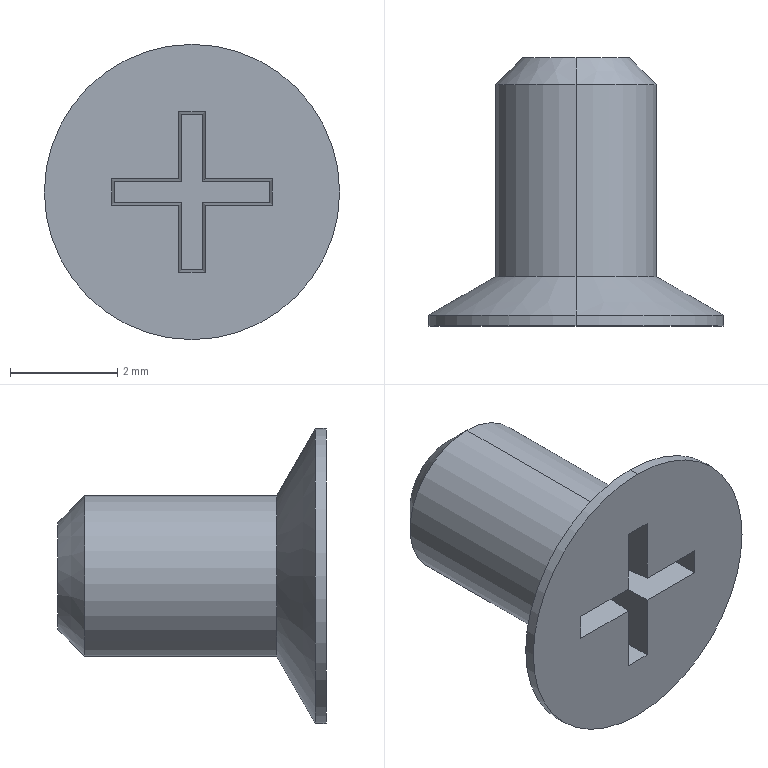Part | SolidWorks | features BaseBody 1 | 1 solid | 23 faces | box 5.5 x 5 x 5.5 mm | volume 40.626 mm3 | plane 15 | cylinder 4 | cone 4 | commonest cylinder face diameters 3 x2 5.5 x2
STEP:
#1=CARTESIAN_POINT('',(0.,0.2,-2.75));
#2=VERTEX_POINT('',#1);
#3=CARTESIAN_POINT('',(0.,0.2,2.75));
#4=VERTEX_POINT('',#3);
#5=CARTESIAN_POINT('',(0.,0.2,0.));
#6=DIRECTION('',(0.,-1.,0.));
#7=DIRECTION('',(0.,0.,-1.));
#8=AXIS2_PLACEMENT_3D('',#5,#6,#7);
#9=CIRCLE('',#8,2.75);
#10=EDGE_CURVE('',#2,#4,#9,.T.);
#11=ORIENTED_EDGE('',*,*,#10,.T.);
#12=CARTESIAN_POINT('',(0.,0.,2.75));
#13=VERTEX_POINT('',#12);
#14=CARTESIAN_POINT('',(0.,0.,2.75));
#15=DIRECTION('',(0.,-1.,0.));
#16=VECTOR('',#15,1000.);
#17=LINE('',#14,#16);
#18=EDGE_CURVE('',#4,#13,#17,.T.);
#19=ORIENTED_EDGE('',*,*,#18,.T.);
#20=CARTESIAN_POINT('',(0.,0.,-2.75));
#21=VERTEX_POINT('',#20);
#22=CARTESIAN_POINT('',(0.,0.,0.));
#23=DIRECTION('',(0.,-1.,0.));
#24=DIRECTION('',(0.,0.,-1.));
#25=AXIS2_PLACEMENT_3D('',#22,#23,#24);
#26=CIRCLE('',#25,2.75);
#27=EDGE_CURVE('',#21,#13,#26,.T.);
#28=ORIENTED_EDGE('',*,*,#27,.F.);
#29=CARTESIAN_POINT('',(0.,0.,-2.75));
#30=DIRECTION('',(0.,-1.,0.));
#31=VECTOR('',#30,1000.);
#32=LINE('',#29,#31);
#33=EDGE_CURVE('',#2,#21,#32,.T.);
#34=ORIENTED_EDGE('',*,*,#33,.F.);
#35=EDGE_LOOP('',(#11,#19,#28,#34));
#36=FACE_OUTER_BOUND('',#35,.T.);
#37=CARTESIAN_POINT('',(0.,0.,0.));
#38=DIRECTION('',(0.,-1.,0.));
#39=DIRECTION('',(0.,0.,-1.));
#40=AXIS2_PLACEMENT_3D('',#37,#38,#39);
#41=CYLINDRICAL_SURFACE('',#40,2.75);
#42=ADVANCED_FACE('',(#36),#41,.T.);
#43=CARTESIAN_POINT('',(0.,0.9217,-1.5));
#44=VERTEX_POINT('',#43);
#45=CARTESIAN_POINT('',(0.,0.9217,1.5));
#46=VERTEX_POINT('',#45);
#47=CARTESIAN_POINT('',(0.,0.9217,0.));
#48=DIRECTION('',(0.,-1.,0.));
#49=DIRECTION('',(0.,0.,-1.));
#50=AXIS2_PLACEMENT_3D('',#47,#48,#49);
#51=CIRCLE('',#50,1.5);
#52=EDGE_CURVE('',#44,#46,#51,.T.);
#53=ORIENTED_EDGE('',*,*,#52,.T.);
#54=CARTESIAN_POINT('',(0.,0.2,2.75));
#55=DIRECTION('',(0.,-0.5,0.866));
#56=VECTOR('',#55,1000.);
#57=LINE('',#54,#56);
#58=EDGE_CURVE('',#46,#4,#57,.T.);
#59=ORIENTED_EDGE('',*,*,#58,.T.);
#60=ORIENTED_EDGE('',*,*,#10,.F.);
#61=CARTESIAN_POINT('',(0.,0.2,-2.75));
#62=DIRECTION('',(0.,-0.5,-0.866));
#63=VECTOR('',#62,1000.);
#64=LINE('',#61,#63);
#65=EDGE_CURVE('',#44,#2,#64,.T.);
#66=ORIENTED_EDGE('',*,*,#65,.F.);
#67=EDGE_LOOP('',(#53,#59,#60,#66));
#68=FACE_OUTER_BOUND('',#67,.T.);
#69=CARTESIAN_POINT('',(0.,0.2,0.));
#70=DIRECTION('',(0.,-1.,0.));
#71=DIRECTION('',(0.,0.,-1.));
#72=AXIS2_PLACEMENT_3D('',#69,#70,#71);
#73=CONICAL_SURFACE('',#72,2.75,1.047);
#74=ADVANCED_FACE('',(#68),#73,.T.);
#75=CARTESIAN_POINT('',(0.,4.5,-1.5));
#76=VERTEX_POINT('',#75);
#77=CARTESIAN_POINT('',(0.,4.5,1.5));
#78=VERTEX_POINT('',#77);
#79=CARTESIAN_POINT('',(0.,4.5,0.));
#80=DIRECTION('',(0.,-1.,0.));
#81=DIRECTION('',(0.,0.,-1.));
#82=AXIS2_PLACEMENT_3D('',#79,#80,#81);
#83=CIRCLE('',#82,1.5);
#84=EDGE_CURVE('',#76,#78,#83,.T.);
#85=ORIENTED_EDGE('',*,*,#84,.T.);
#86=CARTESIAN_POINT('',(0.,0.,1.5));
#87=DIRECTION('',(0.,-1.,0.));
#88=VECTOR('',#87,1000.);
#89=LINE('',#86,#88);
#90=EDGE_CURVE('',#78,#46,#89,.T.);
#91=ORIENTED_EDGE('',*,*,#90,.T.);
#92=ORIENTED_EDGE('',*,*,#52,.F.);
#93=CARTESIAN_POINT('',(0.,0.,-1.5));
#94=DIRECTION('',(0.,-1.,0.));
#95=VECTOR('',#94,1000.);
#96=LINE('',#93,#95);
#97=EDGE_CURVE('',#76,#44,#96,.T.);
#98=ORIENTED_EDGE('',*,*,#97,.F.);
#99=EDGE_LOOP('',(#85,#91,#92,#98));
#100=FACE_OUTER_BOUND('',#99,.T.);
#101=CARTESIAN_POINT('',(0.,0.,0.));
#102=DIRECTION('',(0.,-1.,0.));
#103=DIRECTION('',(0.,0.,-1.));
#104=AXIS2_PLACEMENT_3D('',#101,#102,#103);
#105=CYLINDRICAL_SURFACE('',#104,1.5);
#106=ADVANCED_FACE('',(#100),#105,.T.);
#107=CARTESIAN_POINT('',(0.,5.,-1.));
#108=VERTEX_POINT('',#107);
#109=CARTESIAN_POINT('',(0.,5.,1.));
#110=VERTEX_POINT('',#109);
#111=CARTESIAN_POINT('',(0.,5.,0.));
#112=DIRECTION('',(0.,-1.,0.));
#113=DIRECTION('',(0.,0.,-1.));
#114=AXIS2_PLACEMENT_3D('',#111,#112,#113);
#115=CIRCLE('',#114,1.);
#116=EDGE_CURVE('',#108,#110,#115,.T.);
#117=ORIENTED_EDGE('',*,*,#116,.T.);
#118=CARTESIAN_POINT('',(0.,4.5,1.5));
#119=DIRECTION('',(0.,-0.7071,0.7071));
#120=VECTOR('',#119,1000.);
#121=LINE('',#118,#120);
#122=EDGE_CURVE('',#110,#78,#121,.T.);
#123=ORIENTED_EDGE('',*,*,#122,.T.);
#124=ORIENTED_EDGE('',*,*,#84,.F.);
#125=CARTESIAN_POINT('',(0.,4.5,-1.5));
#126=DIRECTION('',(0.,-0.7071,-0.7071));
#127=VECTOR('',#126,1000.);
#128=LINE('',#125,#127);
#129=EDGE_CURVE('',#108,#76,#128,.T.);
#130=ORIENTED_EDGE('',*,*,#129,.F.);
#131=EDGE_LOOP('',(#117,#123,#124,#130));
#132=FACE_OUTER_BOUND('',#131,.T.);
#133=CARTESIAN_POINT('',(0.,4.5,0.));
#134=DIRECTION('',(0.,-1.,0.));
#135=DIRECTION('',(0.,0.,-1.));
#136=AXIS2_PLACEMENT_3D('',#133,#134,#135);
#137=CONICAL_SURFACE('',#136,1.5,0.7854);
#138=ADVANCED_FACE('',(#132),#137,.T.);
#139=ORIENTED_EDGE('',*,*,#27,.T.);
#140=CARTESIAN_POINT('',(0.,0.,0.));
#141=DIRECTION('',(0.,-1.,0.));
#142=DIRECTION('',(0.,0.,-1.));
#143=AXIS2_PLACEMENT_3D('',#140,#141,#142);
#144=CIRCLE('',#143,2.75);
#145=EDGE_CURVE('',#13,#21,#144,.T.);
#146=ORIENTED_EDGE('',*,*,#145,.T.);
#147=EDGE_LOOP('',(#139,#146));
#148=FACE_OUTER_BOUND('',#147,.T.);
#149=CARTESIAN_POINT('',(-1.5,0.,0.25));
#150=VERTEX_POINT('',#149);
#151=CARTESIAN_POINT('',(-0.25,0.,0.25));
#152=VERTEX_POINT('',#151);
#153=CARTESIAN_POINT('',(2.75,0.,0.25));
#154=DIRECTION('',(1.,0.,0.));
#155=VECTOR('',#154,1000.);
#156=LINE('',#153,#155);
#157=EDGE_CURVE('',#150,#152,#156,.T.);
#158=ORIENTED_EDGE('',*,*,#157,.T.);
#159=CARTESIAN_POINT('',(-0.25,0.,1.5));
#160=VERTEX_POINT('',#159);
#161=CARTESIAN_POINT('',(-0.25,0.,0.));
#162=DIRECTION('',(0.,0.,1.));
#163=VECTOR('',#162,1000.);
#164=LINE('',#161,#163);
#165=EDGE_CURVE('',#152,#160,#164,.T.);
#166=ORIENTED_EDGE('',*,*,#165,.T.);
#167=CARTESIAN_POINT('',(0.25,0.,1.5));
#168=VERTEX_POINT('',#167);
#169=CARTESIAN_POINT('',(2.75,0.,1.5));
#170=DIRECTION('',(1.,0.,0.));
#171=VECTOR('',#170,1000.);
#172=LINE('',#169,#171);
#173=EDGE_CURVE('',#160,#168,#172,.T.);
#174=ORIENTED_EDGE('',*,*,#173,.T.);
#175=CARTESIAN_POINT('',(0.25,0.,0.25));
#176=VERTEX_POINT('',#175);
#177=CARTESIAN_POINT('',(0.25,0.,0.));
#178=DIRECTION('',(0.,0.,-1.));
#179=VECTOR('',#178,1000.);
#180=LINE('',#177,#179);
#181=EDGE_CURVE('',#168,#176,#180,.T.);
#182=ORIENTED_EDGE('',*,*,#181,.T.);
#183=CARTESIAN_POINT('',(1.5,0.,0.25));
#184=VERTEX_POINT('',#183);
#185=CARTESIAN_POINT('',(2.75,0.,0.25));
#186=DIRECTION('',(1.,0.,0.));
#187=VECTOR('',#186,1000.);
#188=LINE('',#185,#187);
#189=EDGE_CURVE('',#176,#184,#188,.T.);
#190=ORIENTED_EDGE('',*,*,#189,.T.);
#191=CARTESIAN_POINT('',(1.5,0.,-0.25));
#192=VERTEX_POINT('',#191);
#193=CARTESIAN_POINT('',(1.5,0.,0.));
#194=DIRECTION('',(0.,0.,-1.));
#195=VECTOR('',#194,1000.);
#196=LINE('',#193,#195);
#197=EDGE_CURVE('',#184,#192,#196,.T.);
#198=ORIENTED_EDGE('',*,*,#197,.T.);
#199=CARTESIAN_POINT('',(0.25,0.,-0.25));
#200=VERTEX_POINT('',#199);
#201=CARTESIAN_POINT('',(2.75,0.,-0.25));
#202=DIRECTION('',(-1.,0.,0.));
#203=VECTOR('',#202,1000.);
#204=LINE('',#201,#203);
#205=EDGE_CURVE('',#192,#200,#204,.T.);
#206=ORIENTED_EDGE('',*,*,#205,.T.);
#207=CARTESIAN_POINT('',(0.25,0.,-1.5));
#208=VERTEX_POINT('',#207);
#209=CARTESIAN_POINT('',(0.25,0.,0.));
#210=DIRECTION('',(0.,0.,-1.));
#211=VECTOR('',#210,1000.);
#212=LINE('',#209,#211);
#213=EDGE_CURVE('',#200,#208,#212,.T.);
#214=ORIENTED_EDGE('',*,*,#213,.T.);
#215=CARTESIAN_POINT('',(-0.25,0.,-1.5));
#216=VERTEX_POINT('',#215);
#217=CARTESIAN_POINT('',(2.75,0.,-1.5));
#218=DIRECTION('',(-1.,0.,0.));
#219=VECTOR('',#218,1000.);
#220=LINE('',#217,#219);
#221=EDGE_CURVE('',#208,#216,#220,.T.);
#222=ORIENTED_EDGE('',*,*,#221,.T.);
#223=CARTESIAN_POINT('',(-0.25,0.,-0.25));
#224=VERTEX_POINT('',#223);
#225=CARTESIAN_POINT('',(-0.25,0.,0.));
#226=DIRECTION('',(0.,0.,1.));
#227=VECTOR('',#226,1000.);
#228=LINE('',#225,#227);
#229=EDGE_CURVE('',#216,#224,#228,.T.);
#230=ORIENTED_EDGE('',*,*,#229,.T.);
#231=CARTESIAN_POINT('',(-1.5,0.,-0.25));
#232=VERTEX_POINT('',#231);
#233=CARTESIAN_POINT('',(2.75,0.,-0.25));
#234=DIRECTION('',(-1.,0.,0.));
#235=VECTOR('',#234,1000.);
#236=LINE('',#233,#235);
#237=EDGE_CURVE('',#224,#232,#236,.T.);
#238=ORIENTED_EDGE('',*,*,#237,.T.);
#239=CARTESIAN_POINT('',(-1.5,0.,0.));
#240=DIRECTION('',(0.,0.,1.));
#241=VECTOR('',#240,1000.);
#242=LINE('',#239,#241);
#243=EDGE_CURVE('',#232,#150,#242,.T.);
#244=ORIENTED_EDGE('',*,*,#243,.T.);
#245=EDGE_LOOP('',(#158,#166,#174,#182,#190,#198,#206,#214,#222,#230,#238,#244));
#246=FACE_BOUND('',#245,.T.);
#247=CARTESIAN_POINT('',(2.75,0.,0.));
#248=DIRECTION('',(0.,-1.,0.));
#249=DIRECTION('',(0.,0.,-1.));
#250=AXIS2_PLACEMENT_3D('',#247,#248,#249);
#251=PLANE('',#250);
#252=ADVANCED_FACE('',(#148,#246),#251,.T.);
#253=ORIENTED_EDGE('',*,*,#18,.F.);
#254=CARTESIAN_POINT('',(0.,0.2,0.));
#255=DIRECTION('',(0.,-1.,0.));
#256=DIRECTION('',(0.,0.,-1.));
#257=AXIS2_PLACEMENT_3D('',#254,#255,#256);
#258=CIRCLE('',#257,2.75);
#259=EDGE_CURVE('',#4,#2,#258,.T.);
#260=ORIENTED_EDGE('',*,*,#259,.T.);
#261=ORIENTED_EDGE('',*,*,#33,.T.);
#262=ORIENTED_EDGE('',*,*,#145,.F.);
#263=EDGE_LOOP('',(#253,#260,#261,#262));
#264=FACE_OUTER_BOUND('',#263,.T.);
#265=CARTESIAN_POINT('',(0.,0.,0.));
#266=DIRECTION('',(0.,-1.,0.));
#267=DIRECTION('',(0.,0.,-1.));
#268=AXIS2_PLACEMENT_3D('',#265,#266,#267);
#269=CYLINDRICAL_SURFACE('',#268,2.75);
#270=ADVANCED_FACE('',(#264),#269,.T.);
#271=CARTESIAN_POINT('',(-0.1976,1.,0.1976));
#272=VERTEX_POINT('',#271);
#273=CARTESIAN_POINT('',(-0.1976,1.,0.1976));
#274=DIRECTION('',(-0.05226,-0.9973,0.05226));
#275=VECTOR('',#274,1000.);
#276=LINE('',#273,#275);
#277=EDGE_CURVE('',#272,#152,#276,.T.);
#278=ORIENTED_EDGE('',*,*,#277,.F.);
#279=CARTESIAN_POINT('',(-0.1976,1.,1.448));
#280=VERTEX_POINT('',#279);
#281=CARTESIAN_POINT('',(-0.1976,1.,0.25));
#282=DIRECTION('',(0.,0.,-1.));
#283=VECTOR('',#282,1000.);
#284=LINE('',#281,#283);
#285=EDGE_CURVE('',#280,#272,#284,.T.);
#286=ORIENTED_EDGE('',*,*,#285,.F.);
#287=CARTESIAN_POINT('',(-0.25,0.,1.5));
#288=DIRECTION('',(0.05226,0.9973,-0.05226));
#289=VECTOR('',#288,1000.);
#290=LINE('',#287,#289);
#291=EDGE_CURVE('',#160,#280,#290,.T.);
#292=ORIENTED_EDGE('',*,*,#291,.F.);
#293=ORIENTED_EDGE('',*,*,#165,.F.);
#294=EDGE_LOOP('',(#278,#286,#292,#293));
#295=FACE_OUTER_BOUND('',#294,.T.);
#296=CARTESIAN_POINT('',(-0.25,0.,0.25));
#297=DIRECTION('',(-0.9986,0.05234,0.));
#298=DIRECTION('',(-0.05234,-0.9986,0.));
#299=AXIS2_PLACEMENT_3D('',#296,#297,#298);
#300=PLANE('',#299);
#301=ADVANCED_FACE('',(#295),#300,.F.);
#302=CARTESIAN_POINT('',(-1.448,1.,0.1976));
#303=VERTEX_POINT('',#302);
#304=CARTESIAN_POINT('',(-1.448,1.,0.1976));
#305=DIRECTION('',(-0.05226,-0.9973,0.05226));
#306=VECTOR('',#305,1000.);
#307=LINE('',#304,#306);
#308=EDGE_CURVE('',#303,#150,#307,.T.);
#309=ORIENTED_EDGE('',*,*,#308,.F.);
#310=CARTESIAN_POINT('',(-1.5,1.,0.1976));
#311=DIRECTION('',(-1.,0.,0.));
#312=VECTOR('',#311,1000.);
#313=LINE('',#310,#312);
#314=EDGE_CURVE('',#272,#303,#313,.T.);
#315=ORIENTED_EDGE('',*,*,#314,.F.);
#316=ORIENTED_EDGE('',*,*,#277,.T.);
#317=ORIENTED_EDGE('',*,*,#157,.F.);
#318=EDGE_LOOP('',(#309,#315,#316,#317));
#319=FACE_OUTER_BOUND('',#318,.T.);
#320=CARTESIAN_POINT('',(-1.5,0.,0.25));
#321=DIRECTION('',(0.,0.05234,0.9986));
#322=DIRECTION('',(0.,-0.9986,0.05234));
#323=AXIS2_PLACEMENT_3D('',#320,#321,#322);
#324=PLANE('',#323);
#325=ADVANCED_FACE('',(#319),#324,.F.);
#326=CARTESIAN_POINT('',(-1.448,1.,-0.1976));
#327=VERTEX_POINT('',#326);
#328=CARTESIAN_POINT('',(-1.448,1.,-0.1976));
#329=DIRECTION('',(-0.05226,-0.9973,-0.05226));
#330=VECTOR('',#329,1000.);
#331=LINE('',#328,#330);
#332=EDGE_CURVE('',#327,#232,#331,.T.);
#333=ORIENTED_EDGE('',*,*,#332,.F.);
#334=CARTESIAN_POINT('',(-1.448,1.,0.25));
#335=DIRECTION('',(0.,0.,-1.));
#336=VECTOR('',#335,1000.);
#337=LINE('',#334,#336);
#338=EDGE_CURVE('',#303,#327,#337,.T.);
#339=ORIENTED_EDGE('',*,*,#338,.F.);
#340=ORIENTED_EDGE('',*,*,#308,.T.);
#341=ORIENTED_EDGE('',*,*,#243,.F.);
#342=EDGE_LOOP('',(#333,#339,#340,#341));
#343=FACE_OUTER_BOUND('',#342,.T.);
#344=CARTESIAN_POINT('',(-1.5,0.,0.25));
#345=DIRECTION('',(-0.9986,0.05234,0.));
#346=DIRECTION('',(-0.05234,-0.9986,0.));
#347=AXIS2_PLACEMENT_3D('',#344,#345,#346);
#348=PLANE('',#347);
#349=ADVANCED_FACE('',(#343),#348,.F.);
#350=CARTESIAN_POINT('',(-0.1976,1.,-0.1976));
#351=VERTEX_POINT('',#350);
#352=CARTESIAN_POINT('',(-0.1976,1.,-0.1976));
#353=DIRECTION('',(-0.05226,-0.9973,-0.05226));
#354=VECTOR('',#353,1000.);
#355=LINE('',#352,#354);
#356=EDGE_CURVE('',#351,#224,#355,.T.);
#357=ORIENTED_EDGE('',*,*,#356,.F.);
#358=CARTESIAN_POINT('',(-1.5,1.,-0.1976));
#359=DIRECTION('',(1.,0.,0.));
#360=VECTOR('',#359,1000.);
#361=LINE('',#358,#360);
#362=EDGE_CURVE('',#327,#351,#361,.T.);
#363=ORIENTED_EDGE('',*,*,#362,.F.);
#364=ORIENTED_EDGE('',*,*,#332,.T.);
#365=ORIENTED_EDGE('',*,*,#237,.F.);
#366=EDGE_LOOP('',(#357,#363,#364,#365));
#367=FACE_OUTER_BOUND('',#366,.T.);
#368=CARTESIAN_POINT('',(-1.5,0.,-0.25));
#369=DIRECTION('',(0.,0.05234,-0.9986));
#370=DIRECTION('',(0.,0.9986,0.05234));
#371=AXIS2_PLACEMENT_3D('',#368,#369,#370);
#372=PLANE('',#371);
#373=ADVANCED_FACE('',(#367),#372,.F.);
#374=CARTESIAN_POINT('',(-0.1976,1.,-1.448));
#375=VERTEX_POINT('',#374);
#376=CARTESIAN_POINT('',(-0.1976,1.,-1.448));
#377=DIRECTION('',(-0.05226,-0.9973,-0.05226));
#378=VECTOR('',#377,1000.);
#379=LINE('',#376,#378);
#380=EDGE_CURVE('',#375,#216,#379,.T.);
#381=ORIENTED_EDGE('',*,*,#380,.F.);
#382=CARTESIAN_POINT('',(-0.1976,1.,-1.5));
#383=DIRECTION('',(0.,0.,-1.));
#384=VECTOR('',#383,1000.);
#385=LINE('',#382,#384);
#386=EDGE_CURVE('',#351,#375,#385,.T.);
#387=ORIENTED_EDGE('',*,*,#386,.F.);
#388=ORIENTED_EDGE('',*,*,#356,.T.);
#389=ORIENTED_EDGE('',*,*,#229,.F.);
#390=EDGE_LOOP('',(#381,#387,#388,#389));
#391=FACE_OUTER_BOUND('',#390,.T.);
#392=CARTESIAN_POINT('',(-0.25,0.,-1.5));
#393=DIRECTION('',(-0.9986,0.05234,0.));
#394=DIRECTION('',(-0.05234,-0.9986,0.));
#395=AXIS2_PLACEMENT_3D('',#392,#393,#394);
#396=PLANE('',#395);
#397=ADVANCED_FACE('',(#391),#396,.F.);
#398=CARTESIAN_POINT('',(0.1976,1.,-1.448));
#399=VERTEX_POINT('',#398);
#400=CARTESIAN_POINT('',(0.1976,1.,-1.448));
#401=DIRECTION('',(0.05226,-0.9973,-0.05226));
#402=VECTOR('',#401,1000.);
#403=LINE('',#400,#402);
#404=EDGE_CURVE('',#399,#208,#403,.T.);
#405=ORIENTED_EDGE('',*,*,#404,.F.);
#406=CARTESIAN_POINT('',(0.25,1.,-1.448));
#407=DIRECTION('',(1.,0.,0.));
#408=VECTOR('',#407,1000.);
#409=LINE('',#406,#408);
#410=EDGE_CURVE('',#375,#399,#409,.T.);
#411=ORIENTED_EDGE('',*,*,#410,.F.);
#412=ORIENTED_EDGE('',*,*,#380,.T.);
#413=ORIENTED_EDGE('',*,*,#221,.F.);
#414=EDGE_LOOP('',(#405,#411,#412,#413));
#415=FACE_OUTER_BOUND('',#414,.T.);
#416=CARTESIAN_POINT('',(0.25,0.,-1.5));
#417=DIRECTION('',(0.,0.05234,-0.9986));
#418=DIRECTION('',(0.,0.9986,0.05234));
#419=AXIS2_PLACEMENT_3D('',#416,#417,#418);
#420=PLANE('',#419);
#421=ADVANCED_FACE('',(#415),#420,.F.);
#422=CARTESIAN_POINT('',(0.1976,1.,-0.1976));
#423=VERTEX_POINT('',#422);
#424=CARTESIAN_POINT('',(0.1976,1.,-0.1976));
#425=DIRECTION('',(0.05226,-0.9973,-0.05226));
#426=VECTOR('',#425,1000.);
#427=LINE('',#424,#426);
#428=EDGE_CURVE('',#423,#200,#427,.T.);
#429=ORIENTED_EDGE('',*,*,#428,.F.);
#430=CARTESIAN_POINT('',(0.1976,1.,-1.5));
#431=DIRECTION('',(0.,0.,1.));
#432=VECTOR('',#431,1000.);
#433=LINE('',#430,#432);
#434=EDGE_CURVE('',#399,#423,#433,.T.);
#435=ORIENTED_EDGE('',*,*,#434,.F.);
#436=ORIENTED_EDGE('',*,*,#404,.T.);
#437=ORIENTED_EDGE('',*,*,#213,.F.);
#438=EDGE_LOOP('',(#429,#435,#436,#437));
#439=FACE_OUTER_BOUND('',#438,.T.);
#440=CARTESIAN_POINT('',(0.25,0.,-1.5));
#441=DIRECTION('',(0.9986,0.05234,0.));
#442=DIRECTION('',(-0.05234,0.9986,0.));
#443=AXIS2_PLACEMENT_3D('',#440,#441,#442);
#444=PLANE('',#443);
#445=ADVANCED_FACE('',(#439),#444,.F.);
#446=CARTESIAN_POINT('',(1.448,1.,-0.1976));
#447=VERTEX_POINT('',#446);
#448=CARTESIAN_POINT('',(1.448,1.,-0.1976));
#449=DIRECTION('',(0.05226,-0.9973,-0.05226));
#450=VECTOR('',#449,1000.);
#451=LINE('',#448,#450);
#452=EDGE_CURVE('',#447,#192,#451,.T.);
#453=ORIENTED_EDGE('',*,*,#452,.F.);
#454=CARTESIAN_POINT('',(0.25,1.,-0.1976));
#455=DIRECTION('',(1.,0.,0.));
#456=VECTOR('',#455,1000.);
#457=LINE('',#454,#456);
#458=EDGE_CURVE('',#423,#447,#457,.T.);
#459=ORIENTED_EDGE('',*,*,#458,.F.);
#460=ORIENTED_EDGE('',*,*,#428,.T.);
#461=ORIENTED_EDGE('',*,*,#205,.F.);
#462=EDGE_LOOP('',(#453,#459,#460,#461));
#463=FACE_OUTER_BOUND('',#462,.T.);
#464=CARTESIAN_POINT('',(0.25,0.,-0.25));
#465=DIRECTION('',(0.,0.05234,-0.9986));
#466=DIRECTION('',(0.,0.9986,0.05234));
#467=AXIS2_PLACEMENT_3D('',#464,#465,#466);
#468=PLANE('',#467);
#469=ADVANCED_FACE('',(#463),#468,.F.);
#470=CARTESIAN_POINT('',(1.448,1.,0.1976));
#471=VERTEX_POINT('',#470);
#472=CARTESIAN_POINT('',(1.448,1.,0.1976));
#473=DIRECTION('',(0.05226,-0.9973,0.05226));
#474=VECTOR('',#473,1000.);
#475=LINE('',#472,#474);
#476=EDGE_CURVE('',#471,#184,#475,.T.);
#477=ORIENTED_EDGE('',*,*,#476,.F.);
#478=CARTESIAN_POINT('',(1.448,1.,0.25));
#479=DIRECTION('',(0.,0.,1.));
#480=VECTOR('',#479,1000.);
#481=LINE('',#478,#480);
#482=EDGE_CURVE('',#447,#471,#481,.T.);
#483=ORIENTED_EDGE('',*,*,#482,.F.);
#484=ORIENTED_EDGE('',*,*,#452,.T.);
#485=ORIENTED_EDGE('',*,*,#197,.F.);
#486=EDGE_LOOP('',(#477,#483,#484,#485));
#487=FACE_OUTER_BOUND('',#486,.T.);
#488=CARTESIAN_POINT('',(1.5,0.,0.25));
#489=DIRECTION('',(0.9986,0.05234,0.));
#490=DIRECTION('',(-0.05234,0.9986,0.));
#491=AXIS2_PLACEMENT_3D('',#488,#489,#490);
#492=PLANE('',#491);
#493=ADVANCED_FACE('',(#487),#492,.F.);
#494=CARTESIAN_POINT('',(0.1976,1.,0.1976));
#495=VERTEX_POINT('',#494);
#496=CARTESIAN_POINT('',(0.1976,1.,0.1976));
#497=DIRECTION('',(0.05226,-0.9973,0.05226));
#498=VECTOR('',#497,1000.);
#499=LINE('',#496,#498);
#500=EDGE_CURVE('',#495,#176,#499,.T.);
#501=ORIENTED_EDGE('',*,*,#500,.F.);
#502=CARTESIAN_POINT('',(0.25,1.,0.1976));
#503=DIRECTION('',(-1.,0.,0.));
#504=VECTOR('',#503,1000.);
#505=LINE('',#502,#504);
#506=EDGE_CURVE('',#471,#495,#505,.T.);
#507=ORIENTED_EDGE('',*,*,#506,.F.);
#508=ORIENTED_EDGE('',*,*,#476,.T.);
#509=ORIENTED_EDGE('',*,*,#189,.F.);
#510=EDGE_LOOP('',(#501,#507,#508,#509));
#511=FACE_OUTER_BOUND('',#510,.T.);
#512=CARTESIAN_POINT('',(0.25,0.,0.25));
#513=DIRECTION('',(0.,0.05234,0.9986));
#514=DIRECTION('',(0.,-0.9986,0.05234));
#515=AXIS2_PLACEMENT_3D('',#512,#513,#514);
#516=PLANE('',#515);
#517=ADVANCED_FACE('',(#511),#516,.F.);
#518=CARTESIAN_POINT('',(0.1976,1.,1.448));
#519=VERTEX_POINT('',#518);
#520=CARTESIAN_POINT('',(0.1976,1.,1.448));
#521=DIRECTION('',(0.05226,-0.9973,0.05226));
#522=VECTOR('',#521,1000.);
#523=LINE('',#520,#522);
#524=EDGE_CURVE('',#519,#168,#523,.T.);
#525=ORIENTED_EDGE('',*,*,#524,.F.);
#526=CARTESIAN_POINT('',(0.1976,1.,0.25));
#527=DIRECTION('',(0.,0.,1.));
#528=VECTOR('',#527,1000.);
#529=LINE('',#526,#528);
#530=EDGE_CURVE('',#495,#519,#529,.T.);
#531=ORIENTED_EDGE('',*,*,#530,.F.);
#532=ORIENTED_EDGE('',*,*,#500,.T.);
#533=ORIENTED_EDGE('',*,*,#181,.F.);
#534=EDGE_LOOP('',(#525,#531,#532,#533));
#535=FACE_OUTER_BOUND('',#534,.T.);
#536=CARTESIAN_POINT('',(0.25,0.,0.25));
#537=DIRECTION('',(0.9986,0.05234,0.));
#538=DIRECTION('',(-0.05234,0.9986,0.));
#539=AXIS2_PLACEMENT_3D('',#536,#537,#538);
#540=PLANE('',#539);
#541=ADVANCED_FACE('',(#535),#540,.F.);
#542=ORIENTED_EDGE('',*,*,#291,.T.);
#543=CARTESIAN_POINT('',(0.25,1.,1.448));
#544=DIRECTION('',(-1.,0.,0.));
#545=VECTOR('',#544,1000.);
#546=LINE('',#543,#545);
#547=EDGE_CURVE('',#519,#280,#546,.T.);
#548=ORIENTED_EDGE('',*,*,#547,.F.);
#549=ORIENTED_EDGE('',*,*,#524,.T.);
#550=ORIENTED_EDGE('',*,*,#173,.F.);
#551=EDGE_LOOP('',(#542,#548,#549,#550));
#552=FACE_OUTER_BOUND('',#551,.T.);
#553=CARTESIAN_POINT('',(0.25,0.,1.5));
#554=DIRECTION('',(0.,0.05234,0.9986));
#555=DIRECTION('',(0.,-0.9986,0.05234));
#556=AXIS2_PLACEMENT_3D('',#553,#554,#555);
#557=PLANE('',#556);
#558=ADVANCED_FACE('',(#552),#557,.F.);
#559=ORIENTED_EDGE('',*,*,#58,.F.);
#560=CARTESIAN_POINT('',(0.,0.9217,0.));
#561=DIRECTION('',(0.,-1.,0.));
#562=DIRECTION('',(0.,0.,-1.));
#563=AXIS2_PLACEMENT_3D('',#560,#561,#562);
#564=CIRCLE('',#563,1.5);
#565=EDGE_CURVE('',#46,#44,#564,.T.);
#566=ORIENTED_EDGE('',*,*,#565,.T.);
#567=ORIENTED_EDGE('',*,*,#65,.T.);
#568=ORIENTED_EDGE('',*,*,#259,.F.);
#569=EDGE_LOOP('',(#559,#566,#567,#568));
#570=FACE_OUTER_BOUND('',#569,.T.);
#571=CARTESIAN_POINT('',(0.,0.2,0.));
#572=DIRECTION('',(0.,-1.,0.));
#573=DIRECTION('',(0.,0.,-1.));
#574=AXIS2_PLACEMENT_3D('',#571,#572,#573);
#575=CONICAL_SURFACE('',#574,2.75,1.047);
#576=ADVANCED_FACE('',(#570),#575,.T.);
#577=ORIENTED_EDGE('',*,*,#285,.T.);
#578=ORIENTED_EDGE('',*,*,#314,.T.);
#579=ORIENTED_EDGE('',*,*,#338,.T.);
#580=ORIENTED_EDGE('',*,*,#362,.T.);
#581=ORIENTED_EDGE('',*,*,#386,.T.);
#582=ORIENTED_EDGE('',*,*,#410,.T.);
#583=ORIENTED_EDGE('',*,*,#434,.T.);
#584=ORIENTED_EDGE('',*,*,#458,.T.);
#585=ORIENTED_EDGE('',*,*,#482,.T.);
#586=ORIENTED_EDGE('',*,*,#506,.T.);
#587=ORIENTED_EDGE('',*,*,#530,.T.);
#588=ORIENTED_EDGE('',*,*,#547,.T.);
#589=EDGE_LOOP('',(#577,#578,#579,#580,#581,#582,#583,#584,#585,#586,#587,#588));
#590=FACE_OUTER_BOUND('',#589,.T.);
#591=CARTESIAN_POINT('',(0.,1.,0.));
#592=DIRECTION('',(0.,1.,0.));
#593=DIRECTION('',(0.,0.,1.));
#594=AXIS2_PLACEMENT_3D('',#591,#592,#593);
#595=PLANE('',#594);
#596=ADVANCED_FACE('',(#590),#595,.F.);
#597=ORIENTED_EDGE('',*,*,#90,.F.);
#598=CARTESIAN_POINT('',(0.,4.5,0.));
#599=DIRECTION('',(0.,-1.,0.));
#600=DIRECTION('',(0.,0.,-1.));
#601=AXIS2_PLACEMENT_3D('',#598,#599,#600);
#602=CIRCLE('',#601,1.5);
#603=EDGE_CURVE('',#78,#76,#602,.T.);
#604=ORIENTED_EDGE('',*,*,#603,.T.);
#605=ORIENTED_EDGE('',*,*,#97,.T.);
#606=ORIENTED_EDGE('',*,*,#565,.F.);
#607=EDGE_LOOP('',(#597,#604,#605,#606));
#608=FACE_OUTER_BOUND('',#607,.T.);
#609=CARTESIAN_POINT('',(0.,0.,0.));
#610=DIRECTION('',(0.,-1.,0.));
#611=DIRECTION('',(0.,0.,-1.));
#612=AXIS2_PLACEMENT_3D('',#609,#610,#611);
#613=CYLINDRICAL_SURFACE('',#612,1.5);
#614=ADVANCED_FACE('',(#608),#613,.T.);
#615=ORIENTED_EDGE('',*,*,#122,.F.);
#616=CARTESIAN_POINT('',(0.,5.,0.));
#617=DIRECTION('',(0.,-1.,0.));
#618=DIRECTION('',(0.,0.,-1.));
#619=AXIS2_PLACEMENT_3D('',#616,#617,#618);
#620=CIRCLE('',#619,1.);
#621=EDGE_CURVE('',#110,#108,#620,.T.);
#622=ORIENTED_EDGE('',*,*,#621,.T.);
#623=ORIENTED_EDGE('',*,*,#129,.T.);
#624=ORIENTED_EDGE('',*,*,#603,.F.);
#625=EDGE_LOOP('',(#615,#622,#623,#624));
#626=FACE_OUTER_BOUND('',#625,.T.);
#627=CARTESIAN_POINT('',(0.,4.5,0.));
#628=DIRECTION('',(0.,-1.,0.));
#629=DIRECTION('',(0.,0.,-1.));
#630=AXIS2_PLACEMENT_3D('',#627,#628,#629);
#631=CONICAL_SURFACE('',#630,1.5,0.7854);
#632=ADVANCED_FACE('',(#626),#631,.T.);
#633=ORIENTED_EDGE('',*,*,#116,.F.);
#634=ORIENTED_EDGE('',*,*,#621,.F.);
#635=EDGE_LOOP('',(#633,#634));
#636=FACE_OUTER_BOUND('',#635,.T.);
#637=CARTESIAN_POINT('',(0.,5.,0.));
#638=DIRECTION('',(0.,1.,0.));
#639=DIRECTION('',(0.,0.,1.));
#640=AXIS2_PLACEMENT_3D('',#637,#638,#639);
#641=PLANE('',#640);
#642=ADVANCED_FACE('',(#636),#641,.T.);
#643=CLOSED_SHELL('',(#42,#74,#106,#138,#252,#270,#301,#325,#349,#373,#397,#421,#445,#469,#493,#517,#541,#558,#576,#596,#614,#632,#642));
#644=MANIFOLD_SOLID_BREP('',#643);
#645=CARTESIAN_POINT('',(0.,0.,0.));
#646=DIRECTION('',(0.,0.,1.));
#647=DIRECTION('',(1.,0.,0.));
#648=AXIS2_PLACEMENT_3D('',#645,#646,#647);
#649=(LENGTH_UNIT()NAMED_UNIT(*)SI_UNIT(.MILLI.,.METRE.));
#650=UNCERTAINTY_MEASURE_WITH_UNIT(LENGTH_MEASURE(0.00001),#649,'','');
#651=(NAMED_UNIT(*)PLANE_ANGLE_UNIT()SI_UNIT($,.RADIAN.));
#652=(NAMED_UNIT(*)SI_UNIT($,.STERADIAN.)SOLID_ANGLE_UNIT());
#653=(GEOMETRIC_REPRESENTATION_CONTEXT(3)GLOBAL_UNCERTAINTY_ASSIGNED_CONTEXT((#650))GLOBAL_UNIT_ASSIGNED_CONTEXT((#649,#651,#652))REPRESENTATION_CONTEXT('',''));
#654=ADVANCED_BREP_SHAPE_REPRESENTATION('',(#644,#648),#653);